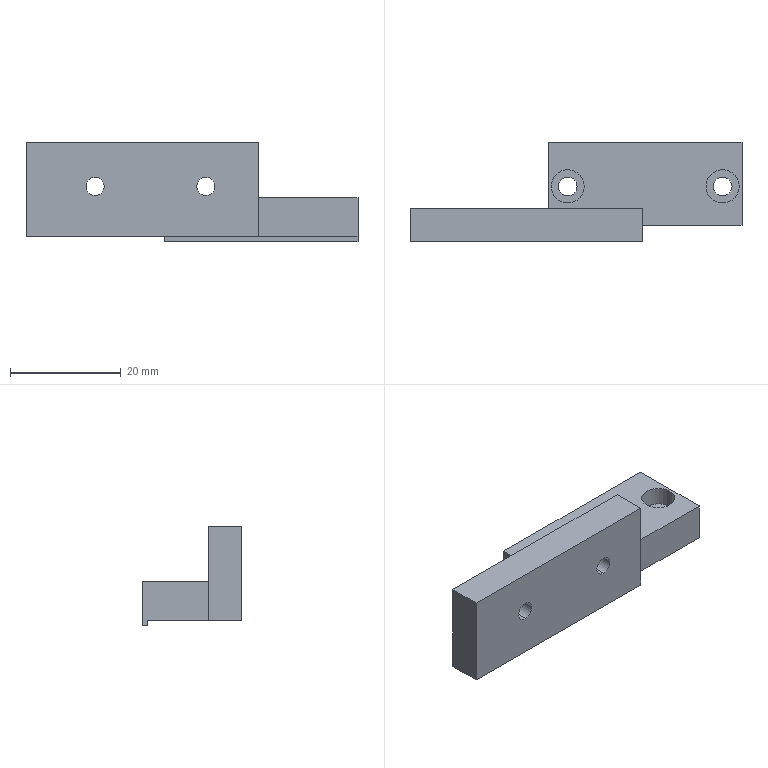Part | STEP file | PN_0026 Mount electronic clip cylinder connecting plate | 1 solid | 27 faces | box 60 x 18 x 18 mm | volume 7277 mm3 | plane 15 | cylinder 12 | commonest cylinder face diameters 3.3 x4 3.4 x4 6 x4